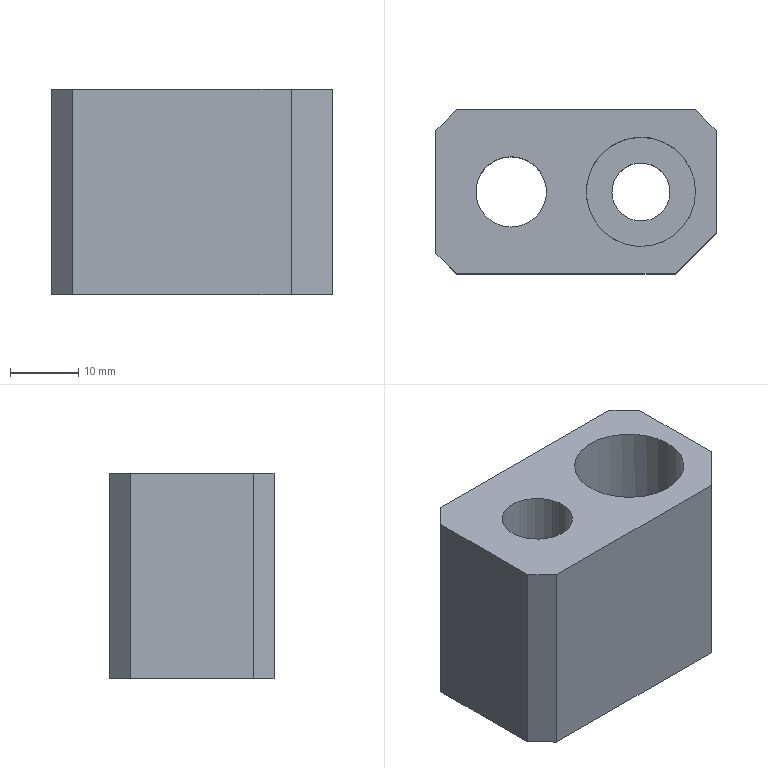Part | NX | features LIN_SOLID_COLOR 2 | 1 solid | 14 faces | box 41 x 24 x 30 mm | volume 22208 mm3 | plane 11 | cylinder 3 | commonest cylinder face diameters 8.5 x1 10.3 x1 16 x1
STEP:
#1=CARTESIAN_POINT('',(-200.,-6.,-31.5));
#2=VERTEX_POINT('',#1);
#3=CARTESIAN_POINT('',(-200.,9.,-31.5));
#4=VERTEX_POINT('',#3);
#5=CARTESIAN_POINT('',(-200.,0.,-31.5));
#6=DIRECTION('',(0.,1.,0.));
#7=VECTOR('',#6,1000.);
#8=LINE('',#5,#7);
#9=EDGE_CURVE('',#2,#4,#8,.T.);
#10=ORIENTED_EDGE('',*,*,#9,.F.);
#11=CARTESIAN_POINT('',(-206.,-12.,-31.5));
#12=VERTEX_POINT('',#11);
#13=CARTESIAN_POINT('',(-208.,-14.,-31.5));
#14=DIRECTION('',(0.7071,0.7071,0.));
#15=VECTOR('',#14,1000.);
#16=LINE('',#13,#15);
#17=EDGE_CURVE('',#2,#12,#16,.F.);
#18=ORIENTED_EDGE('',*,*,#17,.T.);
#19=CARTESIAN_POINT('',(-238.,-12.,-31.5));
#20=VERTEX_POINT('',#19);
#21=CARTESIAN_POINT('',(-223.,-12.,-31.5));
#22=DIRECTION('',(1.,0.,0.));
#23=VECTOR('',#22,1000.);
#24=LINE('',#21,#23);
#25=EDGE_CURVE('',#20,#12,#24,.T.);
#26=ORIENTED_EDGE('',*,*,#25,.F.);
#27=CARTESIAN_POINT('',(-241.,-9.,-31.5));
#28=VERTEX_POINT('',#27);
#29=CARTESIAN_POINT('',(-236.5,-13.5,-31.5));
#30=DIRECTION('',(0.7071,-0.7071,0.));
#31=VECTOR('',#30,1000.);
#32=LINE('',#29,#31);
#33=EDGE_CURVE('',#20,#28,#32,.F.);
#34=ORIENTED_EDGE('',*,*,#33,.T.);
#35=CARTESIAN_POINT('',(-241.,9.,-31.5));
#36=VERTEX_POINT('',#35);
#37=CARTESIAN_POINT('',(-241.,0.,-31.5));
#38=DIRECTION('',(0.,-1.,0.));
#39=VECTOR('',#38,1000.);
#40=LINE('',#37,#39);
#41=EDGE_CURVE('',#36,#28,#40,.T.);
#42=ORIENTED_EDGE('',*,*,#41,.F.);
#43=CARTESIAN_POINT('',(-238.,12.,-31.5));
#44=VERTEX_POINT('',#43);
#45=CARTESIAN_POINT('',(-236.5,13.5,-31.5));
#46=DIRECTION('',(-0.7071,-0.7071,0.));
#47=VECTOR('',#46,1000.);
#48=LINE('',#45,#47);
#49=EDGE_CURVE('',#36,#44,#48,.F.);
#50=ORIENTED_EDGE('',*,*,#49,.T.);
#51=CARTESIAN_POINT('',(-203.,12.,-31.5));
#52=VERTEX_POINT('',#51);
#53=CARTESIAN_POINT('',(-223.,12.,-31.5));
#54=DIRECTION('',(-1.,0.,0.));
#55=VECTOR('',#54,1000.);
#56=LINE('',#53,#55);
#57=EDGE_CURVE('',#52,#44,#56,.T.);
#58=ORIENTED_EDGE('',*,*,#57,.F.);
#59=CARTESIAN_POINT('',(-206.5,15.5,-31.5));
#60=DIRECTION('',(-0.7071,0.7071,0.));
#61=VECTOR('',#60,1000.);
#62=LINE('',#59,#61);
#63=EDGE_CURVE('',#52,#4,#62,.F.);
#64=ORIENTED_EDGE('',*,*,#63,.T.);
#65=EDGE_LOOP('',(#10,#18,#26,#34,#42,#50,#58,#64));
#66=FACE_BOUND('',#65,.T.);
#67=CARTESIAN_POINT('',(-230.,-5.15,-31.5));
#68=VERTEX_POINT('',#67);
#69=CARTESIAN_POINT('',(-230.,0.,-31.5));
#70=DIRECTION('',(0.,0.,-1.));
#71=DIRECTION('',(0.,-1.,0.));
#72=AXIS2_PLACEMENT_3D('',#69,#70,#71);
#73=CIRCLE('',#72,5.15);
#74=EDGE_CURVE('',#68,#68,#73,.T.);
#75=ORIENTED_EDGE('',*,*,#74,.F.);
#76=EDGE_LOOP('',(#75));
#77=FACE_BOUND('',#76,.T.);
#78=CARTESIAN_POINT('',(-215.25,0.,-31.5));
#79=VERTEX_POINT('',#78);
#80=CARTESIAN_POINT('',(-211.,0.,-31.5));
#81=DIRECTION('',(0.,0.,-1.));
#82=DIRECTION('',(-1.,0.,0.));
#83=AXIS2_PLACEMENT_3D('',#80,#81,#82);
#84=CIRCLE('',#83,4.25);
#85=EDGE_CURVE('',#79,#79,#84,.F.);
#86=ORIENTED_EDGE('',*,*,#85,.T.);
#87=EDGE_LOOP('',(#86));
#88=FACE_BOUND('',#87,.T.);
#89=CARTESIAN_POINT('',(-223.,0.,-31.5));
#90=DIRECTION('',(0.,0.,-1.));
#91=DIRECTION('',(-1.,0.,0.));
#92=AXIS2_PLACEMENT_3D('',#89,#90,#91);
#93=PLANE('',#92);
#94=ADVANCED_FACE('',(#66,#77,#88),#93,.T.);
#95=CARTESIAN_POINT('',(-203.,0.,-1.5));
#96=VERTEX_POINT('',#95);
#97=CARTESIAN_POINT('',(-211.,0.,-1.5));
#98=DIRECTION('',(0.,0.,1.));
#99=DIRECTION('',(1.,0.,0.));
#100=AXIS2_PLACEMENT_3D('',#97,#98,#99);
#101=CIRCLE('',#100,8.);
#102=EDGE_CURVE('',#96,#96,#101,.T.);
#103=ORIENTED_EDGE('',*,*,#102,.F.);
#104=EDGE_LOOP('',(#103));
#105=FACE_BOUND('',#104,.T.);
#106=CARTESIAN_POINT('',(-230.,5.15,-1.5));
#107=VERTEX_POINT('',#106);
#108=CARTESIAN_POINT('',(-230.,0.,-1.5));
#109=DIRECTION('',(0.,0.,1.));
#110=DIRECTION('',(0.,1.,0.));
#111=AXIS2_PLACEMENT_3D('',#108,#109,#110);
#112=CIRCLE('',#111,5.15);
#113=EDGE_CURVE('',#107,#107,#112,.T.);
#114=ORIENTED_EDGE('',*,*,#113,.F.);
#115=EDGE_LOOP('',(#114));
#116=FACE_BOUND('',#115,.T.);
#117=CARTESIAN_POINT('',(-206.,-12.,-1.5));
#118=VERTEX_POINT('',#117);
#119=CARTESIAN_POINT('',(-238.,-12.,-1.5));
#120=VERTEX_POINT('',#119);
#121=CARTESIAN_POINT('',(-223.,-12.,-1.5));
#122=DIRECTION('',(-1.,0.,0.));
#123=VECTOR('',#122,1000.);
#124=LINE('',#121,#123);
#125=EDGE_CURVE('',#118,#120,#124,.T.);
#126=ORIENTED_EDGE('',*,*,#125,.F.);
#127=CARTESIAN_POINT('',(-200.,-6.,-1.5));
#128=VERTEX_POINT('',#127);
#129=CARTESIAN_POINT('',(-208.,-14.,-1.5));
#130=DIRECTION('',(-0.7071,-0.7071,0.));
#131=VECTOR('',#130,1000.);
#132=LINE('',#129,#131);
#133=EDGE_CURVE('',#118,#128,#132,.F.);
#134=ORIENTED_EDGE('',*,*,#133,.T.);
#135=CARTESIAN_POINT('',(-200.,9.,-1.5));
#136=VERTEX_POINT('',#135);
#137=CARTESIAN_POINT('',(-200.,0.,-1.5));
#138=DIRECTION('',(0.,-1.,0.));
#139=VECTOR('',#138,1000.);
#140=LINE('',#137,#139);
#141=EDGE_CURVE('',#136,#128,#140,.T.);
#142=ORIENTED_EDGE('',*,*,#141,.F.);
#143=CARTESIAN_POINT('',(-203.,12.,-1.5));
#144=VERTEX_POINT('',#143);
#145=CARTESIAN_POINT('',(-206.5,15.5,-1.5));
#146=DIRECTION('',(0.7071,-0.7071,0.));
#147=VECTOR('',#146,1000.);
#148=LINE('',#145,#147);
#149=EDGE_CURVE('',#136,#144,#148,.F.);
#150=ORIENTED_EDGE('',*,*,#149,.T.);
#151=CARTESIAN_POINT('',(-238.,12.,-1.5));
#152=VERTEX_POINT('',#151);
#153=CARTESIAN_POINT('',(-223.,12.,-1.5));
#154=DIRECTION('',(1.,0.,0.));
#155=VECTOR('',#154,1000.);
#156=LINE('',#153,#155);
#157=EDGE_CURVE('',#152,#144,#156,.T.);
#158=ORIENTED_EDGE('',*,*,#157,.F.);
#159=CARTESIAN_POINT('',(-241.,9.,-1.5));
#160=VERTEX_POINT('',#159);
#161=CARTESIAN_POINT('',(-236.5,13.5,-1.5));
#162=DIRECTION('',(0.7071,0.7071,0.));
#163=VECTOR('',#162,1000.);
#164=LINE('',#161,#163);
#165=EDGE_CURVE('',#152,#160,#164,.F.);
#166=ORIENTED_EDGE('',*,*,#165,.T.);
#167=CARTESIAN_POINT('',(-241.,-9.,-1.5));
#168=VERTEX_POINT('',#167);
#169=CARTESIAN_POINT('',(-241.,0.,-1.5));
#170=DIRECTION('',(0.,1.,0.));
#171=VECTOR('',#170,1000.);
#172=LINE('',#169,#171);
#173=EDGE_CURVE('',#168,#160,#172,.T.);
#174=ORIENTED_EDGE('',*,*,#173,.F.);
#175=CARTESIAN_POINT('',(-236.5,-13.5,-1.5));
#176=DIRECTION('',(-0.7071,0.7071,0.));
#177=VECTOR('',#176,1000.);
#178=LINE('',#175,#177);
#179=EDGE_CURVE('',#168,#120,#178,.F.);
#180=ORIENTED_EDGE('',*,*,#179,.T.);
#181=EDGE_LOOP('',(#126,#134,#142,#150,#158,#166,#174,#180));
#182=FACE_BOUND('',#181,.T.);
#183=CARTESIAN_POINT('',(-223.,0.,-1.5));
#184=DIRECTION('',(0.,0.,1.));
#185=DIRECTION('',(1.,0.,0.));
#186=AXIS2_PLACEMENT_3D('',#183,#184,#185);
#187=PLANE('',#186);
#188=ADVANCED_FACE('',(#105,#116,#182),#187,.T.);
#189=ORIENTED_EDGE('',*,*,#25,.T.);
#190=CARTESIAN_POINT('',(-206.,-12.,-31.5));
#191=DIRECTION('',(0.,0.,1.));
#192=VECTOR('',#191,1000.);
#193=LINE('',#190,#192);
#194=EDGE_CURVE('',#12,#118,#193,.T.);
#195=ORIENTED_EDGE('',*,*,#194,.T.);
#196=ORIENTED_EDGE('',*,*,#125,.T.);
#197=CARTESIAN_POINT('',(-238.,-12.,-31.5));
#198=DIRECTION('',(0.,0.,-1.));
#199=VECTOR('',#198,1000.);
#200=LINE('',#197,#199);
#201=EDGE_CURVE('',#120,#20,#200,.T.);
#202=ORIENTED_EDGE('',*,*,#201,.T.);
#203=EDGE_LOOP('',(#189,#195,#196,#202));
#204=FACE_BOUND('',#203,.T.);
#205=CARTESIAN_POINT('',(-223.,-12.,-31.5));
#206=DIRECTION('',(0.,-1.,0.));
#207=DIRECTION('',(0.,0.,-1.));
#208=AXIS2_PLACEMENT_3D('',#205,#206,#207);
#209=PLANE('',#208);
#210=ADVANCED_FACE('',(#204),#209,.T.);
#211=ORIENTED_EDGE('',*,*,#173,.T.);
#212=CARTESIAN_POINT('',(-241.,9.,-31.5));
#213=DIRECTION('',(0.,0.,-1.));
#214=VECTOR('',#213,1000.);
#215=LINE('',#212,#214);
#216=EDGE_CURVE('',#160,#36,#215,.T.);
#217=ORIENTED_EDGE('',*,*,#216,.T.);
#218=ORIENTED_EDGE('',*,*,#41,.T.);
#219=CARTESIAN_POINT('',(-241.,-9.,-31.5));
#220=DIRECTION('',(0.,0.,1.));
#221=VECTOR('',#220,1000.);
#222=LINE('',#219,#221);
#223=EDGE_CURVE('',#28,#168,#222,.T.);
#224=ORIENTED_EDGE('',*,*,#223,.T.);
#225=EDGE_LOOP('',(#211,#217,#218,#224));
#226=FACE_BOUND('',#225,.T.);
#227=CARTESIAN_POINT('',(-241.,0.,-31.5));
#228=DIRECTION('',(-1.,0.,0.));
#229=DIRECTION('',(0.,0.,1.));
#230=AXIS2_PLACEMENT_3D('',#227,#228,#229);
#231=PLANE('',#230);
#232=ADVANCED_FACE('',(#226),#231,.T.);
#233=ORIENTED_EDGE('',*,*,#157,.T.);
#234=CARTESIAN_POINT('',(-203.,12.,-31.5));
#235=DIRECTION('',(0.,0.,-1.));
#236=VECTOR('',#235,1000.);
#237=LINE('',#234,#236);
#238=EDGE_CURVE('',#144,#52,#237,.T.);
#239=ORIENTED_EDGE('',*,*,#238,.T.);
#240=ORIENTED_EDGE('',*,*,#57,.T.);
#241=CARTESIAN_POINT('',(-238.,12.,-31.5));
#242=DIRECTION('',(0.,0.,1.));
#243=VECTOR('',#242,1000.);
#244=LINE('',#241,#243);
#245=EDGE_CURVE('',#44,#152,#244,.T.);
#246=ORIENTED_EDGE('',*,*,#245,.T.);
#247=EDGE_LOOP('',(#233,#239,#240,#246));
#248=FACE_BOUND('',#247,.T.);
#249=CARTESIAN_POINT('',(-223.,12.,-31.5));
#250=DIRECTION('',(0.,1.,0.));
#251=DIRECTION('',(0.,0.,1.));
#252=AXIS2_PLACEMENT_3D('',#249,#250,#251);
#253=PLANE('',#252);
#254=ADVANCED_FACE('',(#248),#253,.T.);
#255=ORIENTED_EDGE('',*,*,#141,.T.);
#256=CARTESIAN_POINT('',(-200.,-6.,-31.5));
#257=DIRECTION('',(0.,0.,-1.));
#258=VECTOR('',#257,1000.);
#259=LINE('',#256,#258);
#260=EDGE_CURVE('',#128,#2,#259,.T.);
#261=ORIENTED_EDGE('',*,*,#260,.T.);
#262=ORIENTED_EDGE('',*,*,#9,.T.);
#263=CARTESIAN_POINT('',(-200.,9.,-31.5));
#264=DIRECTION('',(0.,0.,1.));
#265=VECTOR('',#264,1000.);
#266=LINE('',#263,#265);
#267=EDGE_CURVE('',#4,#136,#266,.T.);
#268=ORIENTED_EDGE('',*,*,#267,.T.);
#269=EDGE_LOOP('',(#255,#261,#262,#268));
#270=FACE_BOUND('',#269,.T.);
#271=CARTESIAN_POINT('',(-200.,0.,-31.5));
#272=DIRECTION('',(1.,0.,0.));
#273=DIRECTION('',(0.,0.,-1.));
#274=AXIS2_PLACEMENT_3D('',#271,#272,#273);
#275=PLANE('',#274);
#276=ADVANCED_FACE('',(#270),#275,.T.);
#277=ORIENTED_EDGE('',*,*,#113,.T.);
#278=EDGE_LOOP('',(#277));
#279=FACE_BOUND('',#278,.T.);
#280=ORIENTED_EDGE('',*,*,#74,.T.);
#281=EDGE_LOOP('',(#280));
#282=FACE_BOUND('',#281,.T.);
#283=CARTESIAN_POINT('',(-230.,0.,-66.5));
#284=DIRECTION('',(0.,0.,1.));
#285=DIRECTION('',(1.,0.,0.));
#286=AXIS2_PLACEMENT_3D('',#283,#284,#285);
#287=CYLINDRICAL_SURFACE('',#286,5.15);
#288=ADVANCED_FACE('',(#279,#282),#287,.F.);
#289=CARTESIAN_POINT('',(-215.25,0.,-16.5));
#290=VERTEX_POINT('',#289);
#291=CARTESIAN_POINT('',(-211.,0.,-16.5));
#292=DIRECTION('',(0.,0.,-1.));
#293=DIRECTION('',(-1.,0.,0.));
#294=AXIS2_PLACEMENT_3D('',#291,#292,#293);
#295=CIRCLE('',#294,4.25);
#296=EDGE_CURVE('',#290,#290,#295,.F.);
#297=ORIENTED_EDGE('',*,*,#296,.T.);
#298=EDGE_LOOP('',(#297));
#299=FACE_BOUND('',#298,.T.);
#300=ORIENTED_EDGE('',*,*,#85,.F.);
#301=EDGE_LOOP('',(#300));
#302=FACE_BOUND('',#301,.T.);
#303=CARTESIAN_POINT('',(-211.,0.,-31.5));
#304=DIRECTION('',(0.,0.,1.));
#305=DIRECTION('',(1.,0.,0.));
#306=AXIS2_PLACEMENT_3D('',#303,#304,#305);
#307=CYLINDRICAL_SURFACE('',#306,4.25);
#308=ADVANCED_FACE('',(#299,#302),#307,.F.);
#309=CARTESIAN_POINT('',(-219.,0.,-16.5));
#310=VERTEX_POINT('',#309);
#311=CARTESIAN_POINT('',(-211.,0.,-16.5));
#312=DIRECTION('',(0.,0.,-1.));
#313=DIRECTION('',(-1.,0.,0.));
#314=AXIS2_PLACEMENT_3D('',#311,#312,#313);
#315=CIRCLE('',#314,8.);
#316=EDGE_CURVE('',#310,#310,#315,.T.);
#317=ORIENTED_EDGE('',*,*,#316,.F.);
#318=EDGE_LOOP('',(#317));
#319=FACE_BOUND('',#318,.T.);
#320=ORIENTED_EDGE('',*,*,#296,.F.);
#321=EDGE_LOOP('',(#320));
#322=FACE_BOUND('',#321,.T.);
#323=CARTESIAN_POINT('',(-211.,0.,-16.5));
#324=DIRECTION('',(0.,0.,-1.));
#325=DIRECTION('',(-1.,0.,0.));
#326=AXIS2_PLACEMENT_3D('',#323,#324,#325);
#327=PLANE('',#326);
#328=ADVANCED_FACE('',(#319,#322),#327,.F.);
#329=ORIENTED_EDGE('',*,*,#102,.T.);
#330=EDGE_LOOP('',(#329));
#331=FACE_BOUND('',#330,.T.);
#332=ORIENTED_EDGE('',*,*,#316,.T.);
#333=EDGE_LOOP('',(#332));
#334=FACE_BOUND('',#333,.T.);
#335=CARTESIAN_POINT('',(-211.,0.,-11.5));
#336=DIRECTION('',(0.,0.,1.));
#337=DIRECTION('',(1.,0.,0.));
#338=AXIS2_PLACEMENT_3D('',#335,#336,#337);
#339=CYLINDRICAL_SURFACE('',#338,8.);
#340=ADVANCED_FACE('',(#331,#334),#339,.F.);
#341=ORIENTED_EDGE('',*,*,#49,.F.);
#342=ORIENTED_EDGE('',*,*,#216,.F.);
#343=ORIENTED_EDGE('',*,*,#165,.F.);
#344=ORIENTED_EDGE('',*,*,#245,.F.);
#345=EDGE_LOOP('',(#341,#342,#343,#344));
#346=FACE_BOUND('',#345,.T.);
#347=CARTESIAN_POINT('',(-238.,12.,-31.5));
#348=DIRECTION('',(0.7071,-0.7071,0.));
#349=DIRECTION('',(0.,0.,1.));
#350=AXIS2_PLACEMENT_3D('',#347,#348,#349);
#351=PLANE('',#350);
#352=ADVANCED_FACE('',(#346),#351,.F.);
#353=ORIENTED_EDGE('',*,*,#33,.F.);
#354=ORIENTED_EDGE('',*,*,#201,.F.);
#355=ORIENTED_EDGE('',*,*,#179,.F.);
#356=ORIENTED_EDGE('',*,*,#223,.F.);
#357=EDGE_LOOP('',(#353,#354,#355,#356));
#358=FACE_BOUND('',#357,.T.);
#359=CARTESIAN_POINT('',(-241.,-9.,-31.5));
#360=DIRECTION('',(0.7071,0.7071,0.));
#361=DIRECTION('',(0.,0.,1.));
#362=AXIS2_PLACEMENT_3D('',#359,#360,#361);
#363=PLANE('',#362);
#364=ADVANCED_FACE('',(#358),#363,.F.);
#365=ORIENTED_EDGE('',*,*,#149,.F.);
#366=ORIENTED_EDGE('',*,*,#267,.F.);
#367=ORIENTED_EDGE('',*,*,#63,.F.);
#368=ORIENTED_EDGE('',*,*,#238,.F.);
#369=EDGE_LOOP('',(#365,#366,#367,#368));
#370=FACE_BOUND('',#369,.T.);
#371=CARTESIAN_POINT('',(-203.,12.,-31.5));
#372=DIRECTION('',(-0.7071,-0.7071,0.));
#373=DIRECTION('',(0.,0.,-1.));
#374=AXIS2_PLACEMENT_3D('',#371,#372,#373);
#375=PLANE('',#374);
#376=ADVANCED_FACE('',(#370),#375,.F.);
#377=ORIENTED_EDGE('',*,*,#133,.F.);
#378=ORIENTED_EDGE('',*,*,#194,.F.);
#379=ORIENTED_EDGE('',*,*,#17,.F.);
#380=ORIENTED_EDGE('',*,*,#260,.F.);
#381=EDGE_LOOP('',(#377,#378,#379,#380));
#382=FACE_BOUND('',#381,.T.);
#383=CARTESIAN_POINT('',(-200.,-6.,-31.5));
#384=DIRECTION('',(-0.7071,0.7071,0.));
#385=DIRECTION('',(0.,0.,-1.));
#386=AXIS2_PLACEMENT_3D('',#383,#384,#385);
#387=PLANE('',#386);
#388=ADVANCED_FACE('',(#382),#387,.F.);
#389=CLOSED_SHELL('',(#94,#188,#210,#232,#254,#276,#288,#308,#328,#340,#352,#364,#376,#388));
#390=MANIFOLD_SOLID_BREP('',#389);
#391=(LENGTH_UNIT()NAMED_UNIT(*)SI_UNIT(.MILLI.,.METRE.));
#392=UNCERTAINTY_MEASURE_WITH_UNIT(LENGTH_MEASURE(0.00001),#391,'','');
#393=(NAMED_UNIT(*)PLANE_ANGLE_UNIT()SI_UNIT($,.RADIAN.));
#394=(NAMED_UNIT(*)SI_UNIT($,.STERADIAN.)SOLID_ANGLE_UNIT());
#395=(GEOMETRIC_REPRESENTATION_CONTEXT(3)GLOBAL_UNCERTAINTY_ASSIGNED_CONTEXT((#392))GLOBAL_UNIT_ASSIGNED_CONTEXT((#391,#393,#394))REPRESENTATION_CONTEXT('',''));
#396=ADVANCED_BREP_SHAPE_REPRESENTATION('',(#390),#395);